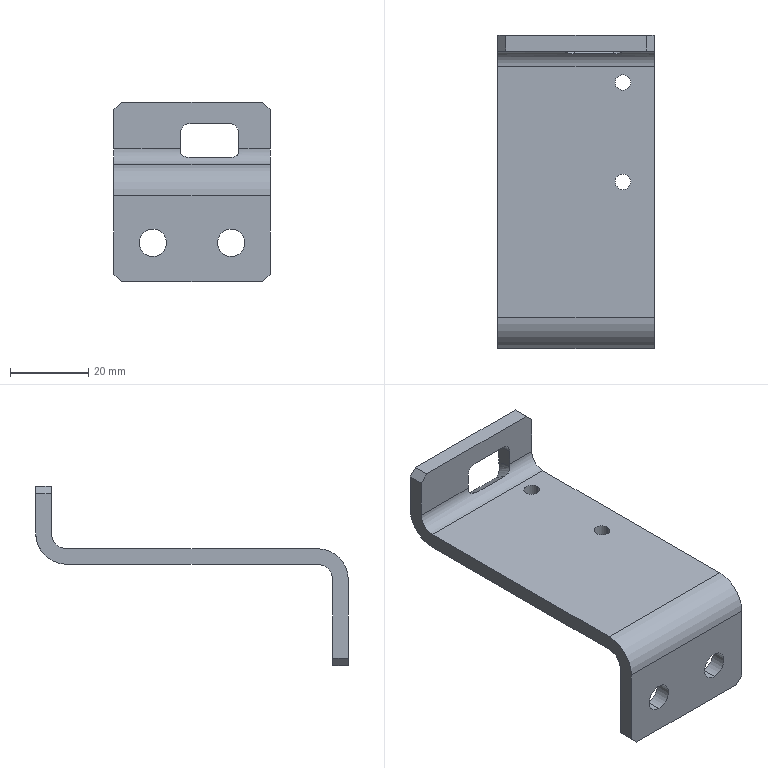Part | STEP file | PN_0028_sensor bracket_default_machined_ | 1 solid | 34 faces | box 40 x 80 x 46 mm | volume 17677 mm3 | plane 18 | cylinder 14 | spline 2 | commonest cylinder face diameters 4 x4 7 x4 5 x2 8 x2 16 x2